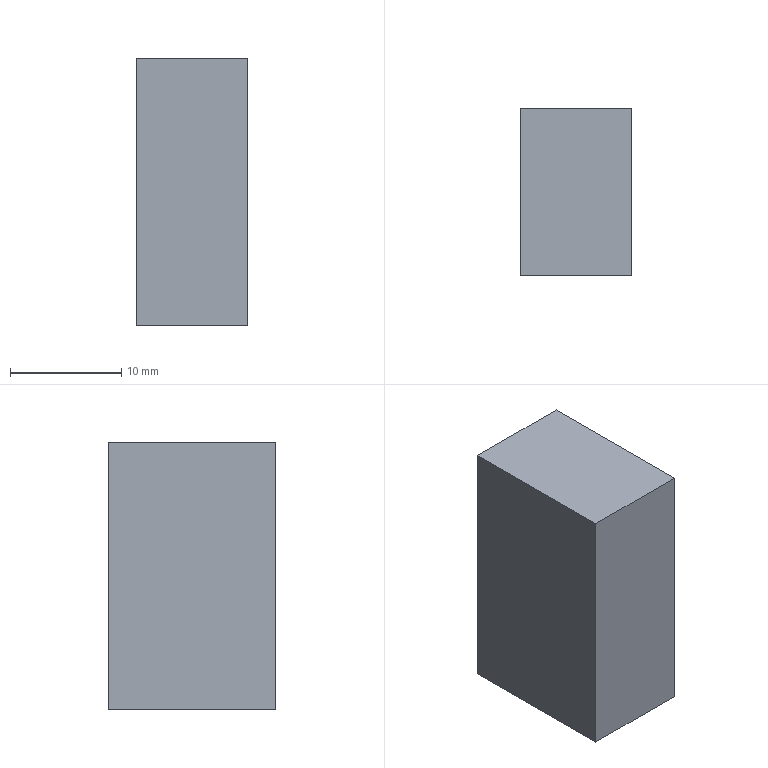Part | NX | features BLOCK 1, DATUM_CSYS 1 | 1 solid | 6 faces | box 10 x 15 x 24 mm | volume 3600 mm3 | plane 6
STEP:
#1=CARTESIAN_POINT('',(10.,0.,24.));
#2=VERTEX_POINT('',#1);
#3=CARTESIAN_POINT('',(0.,0.,24.));
#4=VERTEX_POINT('',#3);
#5=CARTESIAN_POINT('',(5.,0.,24.));
#6=DIRECTION('',(-1.,0.,0.));
#7=VECTOR('',#6,1000.);
#8=LINE('',#5,#7);
#9=EDGE_CURVE('',#2,#4,#8,.T.);
#10=ORIENTED_EDGE('',*,*,#9,.F.);
#11=CARTESIAN_POINT('',(10.,15.,24.));
#12=VERTEX_POINT('',#11);
#13=CARTESIAN_POINT('',(10.,7.5,24.));
#14=DIRECTION('',(0.,-1.,0.));
#15=VECTOR('',#14,1000.);
#16=LINE('',#13,#15);
#17=EDGE_CURVE('',#12,#2,#16,.T.);
#18=ORIENTED_EDGE('',*,*,#17,.F.);
#19=CARTESIAN_POINT('',(0.,15.,24.));
#20=VERTEX_POINT('',#19);
#21=CARTESIAN_POINT('',(5.,15.,24.));
#22=DIRECTION('',(1.,0.,0.));
#23=VECTOR('',#22,1000.);
#24=LINE('',#21,#23);
#25=EDGE_CURVE('',#20,#12,#24,.T.);
#26=ORIENTED_EDGE('',*,*,#25,.F.);
#27=CARTESIAN_POINT('',(0.,7.5,24.));
#28=DIRECTION('',(0.,1.,0.));
#29=VECTOR('',#28,1000.);
#30=LINE('',#27,#29);
#31=EDGE_CURVE('',#4,#20,#30,.T.);
#32=ORIENTED_EDGE('',*,*,#31,.F.);
#33=EDGE_LOOP('',(#10,#18,#26,#32));
#34=FACE_BOUND('',#33,.T.);
#35=CARTESIAN_POINT('',(5.,7.5,24.));
#36=DIRECTION('',(0.,0.,1.));
#37=DIRECTION('',(1.,0.,0.));
#38=AXIS2_PLACEMENT_3D('',#35,#36,#37);
#39=PLANE('',#38);
#40=ADVANCED_FACE('',(#34),#39,.T.);
#41=CARTESIAN_POINT('',(10.,0.,0.));
#42=VERTEX_POINT('',#41);
#43=CARTESIAN_POINT('',(10.,0.,0.));
#44=DIRECTION('',(0.,0.,1.));
#45=VECTOR('',#44,1000.);
#46=LINE('',#43,#45);
#47=EDGE_CURVE('',#42,#2,#46,.T.);
#48=ORIENTED_EDGE('',*,*,#47,.T.);
#49=ORIENTED_EDGE('',*,*,#9,.T.);
#50=CARTESIAN_POINT('',(0.,0.,0.));
#51=VERTEX_POINT('',#50);
#52=CARTESIAN_POINT('',(0.,0.,0.));
#53=DIRECTION('',(0.,0.,1.));
#54=VECTOR('',#53,1000.);
#55=LINE('',#52,#54);
#56=EDGE_CURVE('',#51,#4,#55,.T.);
#57=ORIENTED_EDGE('',*,*,#56,.F.);
#58=CARTESIAN_POINT('',(5.,0.,0.));
#59=DIRECTION('',(1.,0.,0.));
#60=VECTOR('',#59,1000.);
#61=LINE('',#58,#60);
#62=EDGE_CURVE('',#51,#42,#61,.T.);
#63=ORIENTED_EDGE('',*,*,#62,.T.);
#64=EDGE_LOOP('',(#48,#49,#57,#63));
#65=FACE_BOUND('',#64,.T.);
#66=CARTESIAN_POINT('',(5.,0.,0.));
#67=DIRECTION('',(0.,-1.,0.));
#68=DIRECTION('',(0.,0.,-1.));
#69=AXIS2_PLACEMENT_3D('',#66,#67,#68);
#70=PLANE('',#69);
#71=ADVANCED_FACE('',(#65),#70,.T.);
#72=ORIENTED_EDGE('',*,*,#56,.T.);
#73=ORIENTED_EDGE('',*,*,#31,.T.);
#74=CARTESIAN_POINT('',(0.,15.,0.));
#75=VERTEX_POINT('',#74);
#76=CARTESIAN_POINT('',(0.,15.,0.));
#77=DIRECTION('',(0.,0.,1.));
#78=VECTOR('',#77,1000.);
#79=LINE('',#76,#78);
#80=EDGE_CURVE('',#75,#20,#79,.T.);
#81=ORIENTED_EDGE('',*,*,#80,.F.);
#82=CARTESIAN_POINT('',(0.,7.5,0.));
#83=DIRECTION('',(0.,-1.,0.));
#84=VECTOR('',#83,1000.);
#85=LINE('',#82,#84);
#86=EDGE_CURVE('',#75,#51,#85,.T.);
#87=ORIENTED_EDGE('',*,*,#86,.T.);
#88=EDGE_LOOP('',(#72,#73,#81,#87));
#89=FACE_BOUND('',#88,.T.);
#90=CARTESIAN_POINT('',(0.,7.5,0.));
#91=DIRECTION('',(-1.,0.,0.));
#92=DIRECTION('',(0.,0.,1.));
#93=AXIS2_PLACEMENT_3D('',#90,#91,#92);
#94=PLANE('',#93);
#95=ADVANCED_FACE('',(#89),#94,.T.);
#96=ORIENTED_EDGE('',*,*,#80,.T.);
#97=ORIENTED_EDGE('',*,*,#25,.T.);
#98=CARTESIAN_POINT('',(10.,15.,0.));
#99=VERTEX_POINT('',#98);
#100=CARTESIAN_POINT('',(10.,15.,0.));
#101=DIRECTION('',(0.,0.,1.));
#102=VECTOR('',#101,1000.);
#103=LINE('',#100,#102);
#104=EDGE_CURVE('',#99,#12,#103,.T.);
#105=ORIENTED_EDGE('',*,*,#104,.F.);
#106=CARTESIAN_POINT('',(5.,15.,0.));
#107=DIRECTION('',(-1.,0.,0.));
#108=VECTOR('',#107,1000.);
#109=LINE('',#106,#108);
#110=EDGE_CURVE('',#99,#75,#109,.T.);
#111=ORIENTED_EDGE('',*,*,#110,.T.);
#112=EDGE_LOOP('',(#96,#97,#105,#111));
#113=FACE_BOUND('',#112,.T.);
#114=CARTESIAN_POINT('',(5.,15.,0.));
#115=DIRECTION('',(0.,1.,0.));
#116=DIRECTION('',(0.,0.,1.));
#117=AXIS2_PLACEMENT_3D('',#114,#115,#116);
#118=PLANE('',#117);
#119=ADVANCED_FACE('',(#113),#118,.T.);
#120=CARTESIAN_POINT('',(10.,7.5,0.));
#121=DIRECTION('',(0.,1.,0.));
#122=VECTOR('',#121,1000.);
#123=LINE('',#120,#122);
#124=EDGE_CURVE('',#42,#99,#123,.T.);
#125=ORIENTED_EDGE('',*,*,#124,.F.);
#126=ORIENTED_EDGE('',*,*,#62,.F.);
#127=ORIENTED_EDGE('',*,*,#86,.F.);
#128=ORIENTED_EDGE('',*,*,#110,.F.);
#129=EDGE_LOOP('',(#125,#126,#127,#128));
#130=FACE_BOUND('',#129,.T.);
#131=CARTESIAN_POINT('',(5.,7.5,0.));
#132=DIRECTION('',(0.,0.,-1.));
#133=DIRECTION('',(-1.,0.,0.));
#134=AXIS2_PLACEMENT_3D('',#131,#132,#133);
#135=PLANE('',#134);
#136=ADVANCED_FACE('',(#130),#135,.T.);
#137=ORIENTED_EDGE('',*,*,#124,.T.);
#138=ORIENTED_EDGE('',*,*,#104,.T.);
#139=ORIENTED_EDGE('',*,*,#17,.T.);
#140=ORIENTED_EDGE('',*,*,#47,.F.);
#141=EDGE_LOOP('',(#137,#138,#139,#140));
#142=FACE_BOUND('',#141,.T.);
#143=CARTESIAN_POINT('',(10.,7.5,0.));
#144=DIRECTION('',(1.,0.,0.));
#145=DIRECTION('',(0.,0.,-1.));
#146=AXIS2_PLACEMENT_3D('',#143,#144,#145);
#147=PLANE('',#146);
#148=ADVANCED_FACE('',(#142),#147,.T.);
#149=CLOSED_SHELL('',(#40,#71,#95,#119,#136,#148));
#150=MANIFOLD_SOLID_BREP('',#149);
#151=(LENGTH_UNIT()NAMED_UNIT(*)SI_UNIT(.MILLI.,.METRE.));
#152=UNCERTAINTY_MEASURE_WITH_UNIT(LENGTH_MEASURE(0.00001),#151,'','');
#153=(NAMED_UNIT(*)PLANE_ANGLE_UNIT()SI_UNIT($,.RADIAN.));
#154=(NAMED_UNIT(*)SI_UNIT($,.STERADIAN.)SOLID_ANGLE_UNIT());
#155=(GEOMETRIC_REPRESENTATION_CONTEXT(3)GLOBAL_UNCERTAINTY_ASSIGNED_CONTEXT((#152))GLOBAL_UNIT_ASSIGNED_CONTEXT((#151,#153,#154))REPRESENTATION_CONTEXT('',''));
#156=ADVANCED_BREP_SHAPE_REPRESENTATION('',(#150),#155);